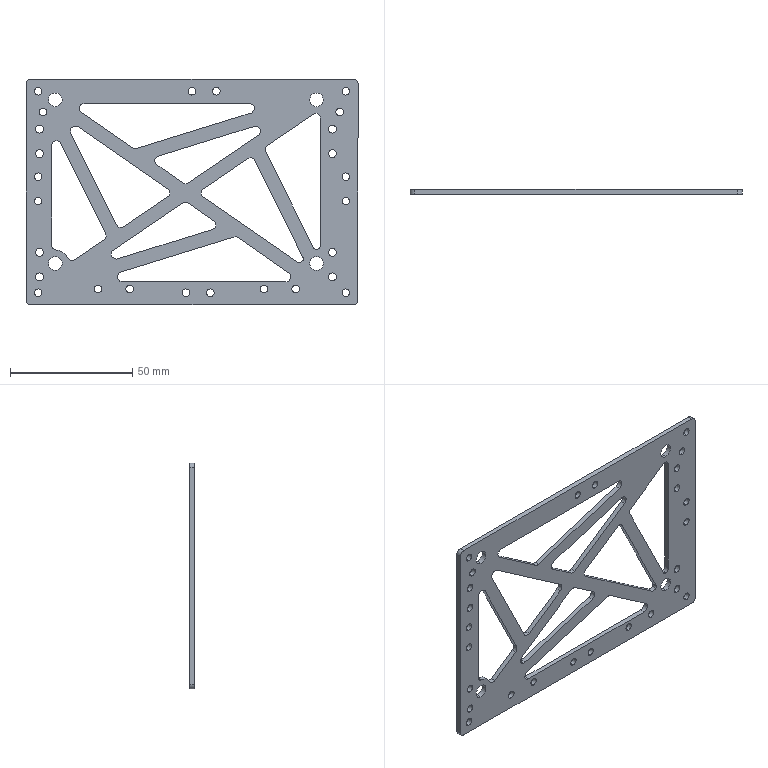Part | SolidWorks | features Fillet 2, Extrusion 1, ICE 1 | 1 solid | 130 faces | box 136 x 2 x 92.5 mm | volume 14381 mm3 | cylinder 100 | plane 30 | commonest cylinder face diameters 4 x36 3.2 x28 3.1 x24 5.6 x8 2 x3 11 x1